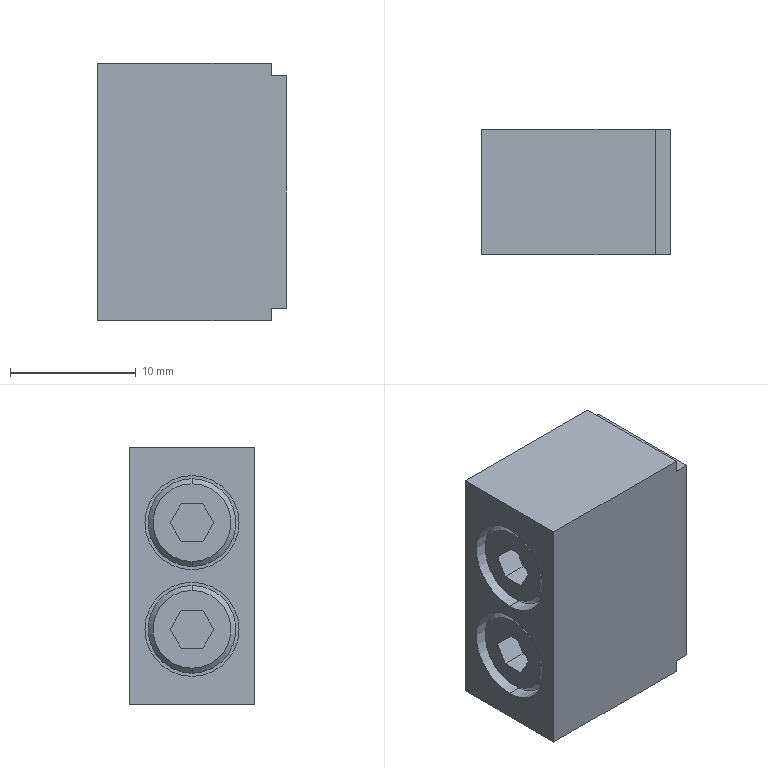Part | SolidWorks | features BaseBody 1 | 1 solid | 40 faces | box 15 x 10 x 20.5 mm | volume 2936 mm3 | plane 28 | cylinder 8 | cone 4 | commonest cylinder face diameters 7 x4 7.5 x4
STEP:
#1=CARTESIAN_POINT('',(-14.6,0.,7.35));
#2=VERTEX_POINT('',#1);
#3=CARTESIAN_POINT('',(-14.6,0.,1.15));
#4=VERTEX_POINT('',#3);
#5=CARTESIAN_POINT('',(-14.6,0.,4.25));
#6=DIRECTION('',(-1.,0.,0.));
#7=DIRECTION('',(0.,0.,1.));
#8=AXIS2_PLACEMENT_3D('',#5,#6,#7);
#9=CIRCLE('',#8,3.1);
#10=EDGE_CURVE('',#2,#4,#9,.T.);
#11=ORIENTED_EDGE('',*,*,#10,.F.);
#12=CARTESIAN_POINT('',(-14.2,0.,7.75));
#13=VERTEX_POINT('',#12);
#14=CARTESIAN_POINT('',(-14.2,0.,7.75));
#15=DIRECTION('',(0.7071,0.,0.7071));
#16=VECTOR('',#15,1000.);
#17=LINE('',#14,#16);
#18=EDGE_CURVE('',#2,#13,#17,.T.);
#19=ORIENTED_EDGE('',*,*,#18,.T.);
#20=CARTESIAN_POINT('',(-14.2,0.,0.75));
#21=VERTEX_POINT('',#20);
#22=CARTESIAN_POINT('',(-14.2,0.,4.25));
#23=DIRECTION('',(-1.,0.,0.));
#24=DIRECTION('',(0.,0.,1.));
#25=AXIS2_PLACEMENT_3D('',#22,#23,#24);
#26=CIRCLE('',#25,3.5);
#27=EDGE_CURVE('',#13,#21,#26,.T.);
#28=ORIENTED_EDGE('',*,*,#27,.T.);
#29=CARTESIAN_POINT('',(-14.2,0.,0.75));
#30=DIRECTION('',(0.7071,0.,-0.7071));
#31=VECTOR('',#30,1000.);
#32=LINE('',#29,#31);
#33=EDGE_CURVE('',#4,#21,#32,.T.);
#34=ORIENTED_EDGE('',*,*,#33,.F.);
#35=EDGE_LOOP('',(#11,#19,#28,#34));
#36=FACE_OUTER_BOUND('',#35,.T.);
#37=CARTESIAN_POINT('',(-14.2,0.,4.25));
#38=DIRECTION('',(1.,0.,0.));
#39=DIRECTION('',(0.,0.,-1.));
#40=AXIS2_PLACEMENT_3D('',#37,#38,#39);
#41=CONICAL_SURFACE('',#40,3.5,0.7854);
#42=ADVANCED_FACE('',(#36),#41,.T.);
#43=CARTESIAN_POINT('',(-10.6,0.,7.75));
#44=VERTEX_POINT('',#43);
#45=CARTESIAN_POINT('',(-10.6,0.,0.75));
#46=VERTEX_POINT('',#45);
#47=CARTESIAN_POINT('',(-10.6,0.,4.25));
#48=DIRECTION('',(-1.,0.,0.));
#49=DIRECTION('',(0.,0.,-1.));
#50=AXIS2_PLACEMENT_3D('',#47,#48,#49);
#51=CIRCLE('',#50,3.5);
#52=EDGE_CURVE('',#44,#46,#51,.T.);
#53=ORIENTED_EDGE('',*,*,#52,.T.);
#54=CARTESIAN_POINT('',(-14.6,0.,0.75));
#55=DIRECTION('',(-1.,0.,0.));
#56=VECTOR('',#55,1000.);
#57=LINE('',#54,#56);
#58=EDGE_CURVE('',#46,#21,#57,.T.);
#59=ORIENTED_EDGE('',*,*,#58,.T.);
#60=ORIENTED_EDGE('',*,*,#27,.F.);
#61=CARTESIAN_POINT('',(-14.6,0.,7.75));
#62=DIRECTION('',(-1.,0.,0.));
#63=VECTOR('',#62,1000.);
#64=LINE('',#61,#63);
#65=EDGE_CURVE('',#44,#13,#64,.T.);
#66=ORIENTED_EDGE('',*,*,#65,.F.);
#67=EDGE_LOOP('',(#53,#59,#60,#66));
#68=FACE_OUTER_BOUND('',#67,.T.);
#69=CARTESIAN_POINT('',(-14.6,0.,4.25));
#70=DIRECTION('',(-1.,0.,0.));
#71=DIRECTION('',(0.,0.,1.));
#72=AXIS2_PLACEMENT_3D('',#69,#70,#71);
#73=CYLINDRICAL_SURFACE('',#72,3.5);
#74=ADVANCED_FACE('',(#68),#73,.T.);
#75=CARTESIAN_POINT('',(-10.6,0.,8.));
#76=VERTEX_POINT('',#75);
#77=CARTESIAN_POINT('',(-10.6,0.,0.5));
#78=VERTEX_POINT('',#77);
#79=CARTESIAN_POINT('',(-10.6,0.,4.25));
#80=DIRECTION('',(1.,0.,0.));
#81=DIRECTION('',(0.,0.,-1.));
#82=AXIS2_PLACEMENT_3D('',#79,#80,#81);
#83=CIRCLE('',#82,3.75);
#84=EDGE_CURVE('',#76,#78,#83,.T.);
#85=ORIENTED_EDGE('',*,*,#84,.T.);
#86=CARTESIAN_POINT('',(-15.,0.,0.5));
#87=VERTEX_POINT('',#86);
#88=CARTESIAN_POINT('',(-10.6,0.,0.5));
#89=DIRECTION('',(-1.,0.,0.));
#90=VECTOR('',#89,1000.);
#91=LINE('',#88,#90);
#92=EDGE_CURVE('',#78,#87,#91,.T.);
#93=ORIENTED_EDGE('',*,*,#92,.T.);
#94=CARTESIAN_POINT('',(-15.,0.,8.));
#95=VERTEX_POINT('',#94);
#96=CARTESIAN_POINT('',(-15.,0.,4.25));
#97=DIRECTION('',(1.,0.,0.));
#98=DIRECTION('',(0.,0.,-1.));
#99=AXIS2_PLACEMENT_3D('',#96,#97,#98);
#100=CIRCLE('',#99,3.75);
#101=EDGE_CURVE('',#95,#87,#100,.T.);
#102=ORIENTED_EDGE('',*,*,#101,.F.);
#103=CARTESIAN_POINT('',(-10.6,0.,8.));
#104=DIRECTION('',(-1.,0.,0.));
#105=VECTOR('',#104,1000.);
#106=LINE('',#103,#105);
#107=EDGE_CURVE('',#76,#95,#106,.T.);
#108=ORIENTED_EDGE('',*,*,#107,.F.);
#109=EDGE_LOOP('',(#85,#93,#102,#108));
#110=FACE_OUTER_BOUND('',#109,.T.);
#111=CARTESIAN_POINT('',(-10.6,0.,4.25));
#112=DIRECTION('',(-1.,0.,0.));
#113=DIRECTION('',(0.,0.,1.));
#114=AXIS2_PLACEMENT_3D('',#111,#112,#113);
#115=CYLINDRICAL_SURFACE('',#114,3.75);
#116=ADVANCED_FACE('',(#110),#115,.F.);
#117=CARTESIAN_POINT('',(-10.6,0.,-0.5));
#118=VERTEX_POINT('',#117);
#119=CARTESIAN_POINT('',(-10.6,0.,-8.));
#120=VERTEX_POINT('',#119);
#121=CARTESIAN_POINT('',(-10.6,0.,-4.25));
#122=DIRECTION('',(1.,0.,0.));
#123=DIRECTION('',(0.,0.,-1.));
#124=AXIS2_PLACEMENT_3D('',#121,#122,#123);
#125=CIRCLE('',#124,3.75);
#126=EDGE_CURVE('',#118,#120,#125,.T.);
#127=ORIENTED_EDGE('',*,*,#126,.T.);
#128=CARTESIAN_POINT('',(-15.,0.,-8.));
#129=VERTEX_POINT('',#128);
#130=CARTESIAN_POINT('',(-10.6,0.,-8.));
#131=DIRECTION('',(-1.,0.,0.));
#132=VECTOR('',#131,1000.);
#133=LINE('',#130,#132);
#134=EDGE_CURVE('',#120,#129,#133,.T.);
#135=ORIENTED_EDGE('',*,*,#134,.T.);
#136=CARTESIAN_POINT('',(-15.,0.,-0.5));
#137=VERTEX_POINT('',#136);
#138=CARTESIAN_POINT('',(-15.,0.,-4.25));
#139=DIRECTION('',(1.,0.,0.));
#140=DIRECTION('',(0.,0.,-1.));
#141=AXIS2_PLACEMENT_3D('',#138,#139,#140);
#142=CIRCLE('',#141,3.75);
#143=EDGE_CURVE('',#137,#129,#142,.T.);
#144=ORIENTED_EDGE('',*,*,#143,.F.);
#145=CARTESIAN_POINT('',(-10.6,0.,-0.5));
#146=DIRECTION('',(-1.,0.,0.));
#147=VECTOR('',#146,1000.);
#148=LINE('',#145,#147);
#149=EDGE_CURVE('',#118,#137,#148,.T.);
#150=ORIENTED_EDGE('',*,*,#149,.F.);
#151=EDGE_LOOP('',(#127,#135,#144,#150));
#152=FACE_OUTER_BOUND('',#151,.T.);
#153=CARTESIAN_POINT('',(-10.6,0.,-4.25));
#154=DIRECTION('',(-1.,0.,0.));
#155=DIRECTION('',(0.,0.,1.));
#156=AXIS2_PLACEMENT_3D('',#153,#154,#155);
#157=CYLINDRICAL_SURFACE('',#156,3.75);
#158=ADVANCED_FACE('',(#152),#157,.F.);
#159=CARTESIAN_POINT('',(-10.6,0.,-0.75));
#160=VERTEX_POINT('',#159);
#161=CARTESIAN_POINT('',(-10.6,0.,-7.75));
#162=VERTEX_POINT('',#161);
#163=CARTESIAN_POINT('',(-10.6,0.,-4.25));
#164=DIRECTION('',(-1.,0.,0.));
#165=DIRECTION('',(0.,0.,-1.));
#166=AXIS2_PLACEMENT_3D('',#163,#164,#165);
#167=CIRCLE('',#166,3.5);
#168=EDGE_CURVE('',#160,#162,#167,.T.);
#169=ORIENTED_EDGE('',*,*,#168,.T.);
#170=CARTESIAN_POINT('',(-14.2,0.,-7.75));
#171=VERTEX_POINT('',#170);
#172=CARTESIAN_POINT('',(-14.6,0.,-7.75));
#173=DIRECTION('',(-1.,0.,0.));
#174=VECTOR('',#173,1000.);
#175=LINE('',#172,#174);
#176=EDGE_CURVE('',#162,#171,#175,.T.);
#177=ORIENTED_EDGE('',*,*,#176,.T.);
#178=CARTESIAN_POINT('',(-14.2,0.,-0.75));
#179=VERTEX_POINT('',#178);
#180=CARTESIAN_POINT('',(-14.2,0.,-4.25));
#181=DIRECTION('',(-1.,0.,0.));
#182=DIRECTION('',(0.,0.,1.));
#183=AXIS2_PLACEMENT_3D('',#180,#181,#182);
#184=CIRCLE('',#183,3.5);
#185=EDGE_CURVE('',#179,#171,#184,.T.);
#186=ORIENTED_EDGE('',*,*,#185,.F.);
#187=CARTESIAN_POINT('',(-14.6,0.,-0.75));
#188=DIRECTION('',(-1.,0.,0.));
#189=VECTOR('',#188,1000.);
#190=LINE('',#187,#189);
#191=EDGE_CURVE('',#160,#179,#190,.T.);
#192=ORIENTED_EDGE('',*,*,#191,.F.);
#193=EDGE_LOOP('',(#169,#177,#186,#192));
#194=FACE_OUTER_BOUND('',#193,.T.);
#195=CARTESIAN_POINT('',(-14.6,0.,-4.25));
#196=DIRECTION('',(-1.,0.,0.));
#197=DIRECTION('',(0.,0.,1.));
#198=AXIS2_PLACEMENT_3D('',#195,#196,#197);
#199=CYLINDRICAL_SURFACE('',#198,3.5);
#200=ADVANCED_FACE('',(#194),#199,.T.);
#201=CARTESIAN_POINT('',(-14.6,0.,-1.15));
#202=VERTEX_POINT('',#201);
#203=CARTESIAN_POINT('',(-14.6,0.,-7.35));
#204=VERTEX_POINT('',#203);
#205=CARTESIAN_POINT('',(-14.6,0.,-4.25));
#206=DIRECTION('',(-1.,0.,0.));
#207=DIRECTION('',(0.,0.,1.));
#208=AXIS2_PLACEMENT_3D('',#205,#206,#207);
#209=CIRCLE('',#208,3.1);
#210=EDGE_CURVE('',#202,#204,#209,.T.);
#211=ORIENTED_EDGE('',*,*,#210,.F.);
#212=CARTESIAN_POINT('',(-14.2,0.,-0.75));
#213=DIRECTION('',(0.7071,0.,0.7071));
#214=VECTOR('',#213,1000.);
#215=LINE('',#212,#214);
#216=EDGE_CURVE('',#202,#179,#215,.T.);
#217=ORIENTED_EDGE('',*,*,#216,.T.);
#218=ORIENTED_EDGE('',*,*,#185,.T.);
#219=CARTESIAN_POINT('',(-14.2,0.,-7.75));
#220=DIRECTION('',(0.7071,0.,-0.7071));
#221=VECTOR('',#220,1000.);
#222=LINE('',#219,#221);
#223=EDGE_CURVE('',#204,#171,#222,.T.);
#224=ORIENTED_EDGE('',*,*,#223,.F.);
#225=EDGE_LOOP('',(#211,#217,#218,#224));
#226=FACE_OUTER_BOUND('',#225,.T.);
#227=CARTESIAN_POINT('',(-14.2,0.,-4.25));
#228=DIRECTION('',(1.,0.,0.));
#229=DIRECTION('',(0.,0.,-1.));
#230=AXIS2_PLACEMENT_3D('',#227,#228,#229);
#231=CONICAL_SURFACE('',#230,3.5,0.7854);
#232=ADVANCED_FACE('',(#226),#231,.T.);
#233=CARTESIAN_POINT('',(-14.6,1.732,-4.25));
#234=VERTEX_POINT('',#233);
#235=CARTESIAN_POINT('',(-14.6,0.866,-2.75));
#236=VERTEX_POINT('',#235);
#237=CARTESIAN_POINT('',(-14.6,1.732,-4.25));
#238=DIRECTION('',(0.,-0.5,0.866));
#239=VECTOR('',#238,1000.);
#240=LINE('',#237,#239);
#241=EDGE_CURVE('',#234,#236,#240,.T.);
#242=ORIENTED_EDGE('',*,*,#241,.T.);
#243=CARTESIAN_POINT('',(-14.6,-0.866,-2.75));
#244=VERTEX_POINT('',#243);
#245=CARTESIAN_POINT('',(-14.6,-0.866,-2.75));
#246=DIRECTION('',(0.,1.,0.));
#247=VECTOR('',#246,1000.);
#248=LINE('',#245,#247);
#249=EDGE_CURVE('',#244,#236,#248,.T.);
#250=ORIENTED_EDGE('',*,*,#249,.F.);
#251=CARTESIAN_POINT('',(-14.6,-1.732,-4.25));
#252=VERTEX_POINT('',#251);
#253=CARTESIAN_POINT('',(-14.6,-0.866,-2.75));
#254=DIRECTION('',(0.,-0.5,-0.866));
#255=VECTOR('',#254,1000.);
#256=LINE('',#253,#255);
#257=EDGE_CURVE('',#244,#252,#256,.T.);
#258=ORIENTED_EDGE('',*,*,#257,.T.);
#259=CARTESIAN_POINT('',(-14.6,-0.866,-5.75));
#260=VERTEX_POINT('',#259);
#261=CARTESIAN_POINT('',(-14.6,-1.732,-4.25));
#262=DIRECTION('',(0.,0.5,-0.866));
#263=VECTOR('',#262,1000.);
#264=LINE('',#261,#263);
#265=EDGE_CURVE('',#252,#260,#264,.T.);
#266=ORIENTED_EDGE('',*,*,#265,.T.);
#267=CARTESIAN_POINT('',(-14.6,0.866,-5.75));
#268=VERTEX_POINT('',#267);
#269=CARTESIAN_POINT('',(-14.6,-0.866,-5.75));
#270=DIRECTION('',(0.,1.,0.));
#271=VECTOR('',#270,1000.);
#272=LINE('',#269,#271);
#273=EDGE_CURVE('',#260,#268,#272,.T.);
#274=ORIENTED_EDGE('',*,*,#273,.T.);
#275=CARTESIAN_POINT('',(-14.6,0.866,-5.75));
#276=DIRECTION('',(0.,0.5,0.866));
#277=VECTOR('',#276,1000.);
#278=LINE('',#275,#277);
#279=EDGE_CURVE('',#268,#234,#278,.T.);
#280=ORIENTED_EDGE('',*,*,#279,.T.);
#281=EDGE_LOOP('',(#242,#250,#258,#266,#274,#280));
#282=FACE_BOUND('',#281,.T.);
#283=CARTESIAN_POINT('',(-14.6,0.,-4.25));
#284=DIRECTION('',(-1.,0.,0.));
#285=DIRECTION('',(0.,0.,1.));
#286=AXIS2_PLACEMENT_3D('',#283,#284,#285);
#287=CIRCLE('',#286,3.1);
#288=EDGE_CURVE('',#204,#202,#287,.T.);
#289=ORIENTED_EDGE('',*,*,#288,.T.);
#290=ORIENTED_EDGE('',*,*,#210,.T.);
#291=EDGE_LOOP('',(#289,#290));
#292=FACE_OUTER_BOUND('',#291,.T.);
#293=CARTESIAN_POINT('',(-14.6,0.,-1.15));
#294=DIRECTION('',(1.,0.,0.));
#295=DIRECTION('',(0.,0.,-1.));
#296=AXIS2_PLACEMENT_3D('',#293,#294,#295);
#297=PLANE('',#296);
#298=ADVANCED_FACE('',(#282,#292),#297,.F.);
#299=ORIENTED_EDGE('',*,*,#241,.F.);
#300=CARTESIAN_POINT('',(-12.6,1.732,-4.25));
#301=VERTEX_POINT('',#300);
#302=CARTESIAN_POINT('',(-12.6,1.732,-4.25));
#303=DIRECTION('',(-1.,0.,0.));
#304=VECTOR('',#303,1000.);
#305=LINE('',#302,#304);
#306=EDGE_CURVE('',#301,#234,#305,.T.);
#307=ORIENTED_EDGE('',*,*,#306,.F.);
#308=CARTESIAN_POINT('',(-12.6,0.866,-2.75));
#309=VERTEX_POINT('',#308);
#310=CARTESIAN_POINT('',(-12.6,1.732,-4.25));
#311=DIRECTION('',(0.,-0.5,0.866));
#312=VECTOR('',#311,1000.);
#313=LINE('',#310,#312);
#314=EDGE_CURVE('',#301,#309,#313,.T.);
#315=ORIENTED_EDGE('',*,*,#314,.T.);
#316=CARTESIAN_POINT('',(-12.6,0.866,-2.75));
#317=DIRECTION('',(-1.,0.,0.));
#318=VECTOR('',#317,1000.);
#319=LINE('',#316,#318);
#320=EDGE_CURVE('',#309,#236,#319,.T.);
#321=ORIENTED_EDGE('',*,*,#320,.T.);
#322=EDGE_LOOP('',(#299,#307,#315,#321));
#323=FACE_OUTER_BOUND('',#322,.T.);
#324=CARTESIAN_POINT('',(-12.6,1.732,-4.25));
#325=DIRECTION('',(0.,-0.866,-0.5));
#326=DIRECTION('',(0.,0.5,-0.866));
#327=AXIS2_PLACEMENT_3D('',#324,#325,#326);
#328=PLANE('',#327);
#329=ADVANCED_FACE('',(#323),#328,.T.);
#330=ORIENTED_EDGE('',*,*,#249,.T.);
#331=ORIENTED_EDGE('',*,*,#320,.F.);
#332=CARTESIAN_POINT('',(-12.6,-0.866,-2.75));
#333=VERTEX_POINT('',#332);
#334=CARTESIAN_POINT('',(-12.6,0.866,-2.75));
#335=DIRECTION('',(0.,-1.,0.));
#336=VECTOR('',#335,1000.);
#337=LINE('',#334,#336);
#338=EDGE_CURVE('',#309,#333,#337,.T.);
#339=ORIENTED_EDGE('',*,*,#338,.T.);
#340=CARTESIAN_POINT('',(-12.6,-0.866,-2.75));
#341=DIRECTION('',(-1.,0.,0.));
#342=VECTOR('',#341,1000.);
#343=LINE('',#340,#342);
#344=EDGE_CURVE('',#333,#244,#343,.T.);
#345=ORIENTED_EDGE('',*,*,#344,.T.);
#346=EDGE_LOOP('',(#330,#331,#339,#345));
#347=FACE_OUTER_BOUND('',#346,.T.);
#348=CARTESIAN_POINT('',(-12.6,0.866,-2.75));
#349=DIRECTION('',(0.,0.,-1.));
#350=DIRECTION('',(-1.,0.,0.));
#351=AXIS2_PLACEMENT_3D('',#348,#349,#350);
#352=PLANE('',#351);
#353=ADVANCED_FACE('',(#347),#352,.T.);
#354=ORIENTED_EDGE('',*,*,#257,.F.);
#355=ORIENTED_EDGE('',*,*,#344,.F.);
#356=CARTESIAN_POINT('',(-12.6,-1.732,-4.25));
#357=VERTEX_POINT('',#356);
#358=CARTESIAN_POINT('',(-12.6,-0.866,-2.75));
#359=DIRECTION('',(0.,-0.5,-0.866));
#360=VECTOR('',#359,1000.);
#361=LINE('',#358,#360);
#362=EDGE_CURVE('',#333,#357,#361,.T.);
#363=ORIENTED_EDGE('',*,*,#362,.T.);
#364=CARTESIAN_POINT('',(-12.6,-1.732,-4.25));
#365=DIRECTION('',(-1.,0.,0.));
#366=VECTOR('',#365,1000.);
#367=LINE('',#364,#366);
#368=EDGE_CURVE('',#357,#252,#367,.T.);
#369=ORIENTED_EDGE('',*,*,#368,.T.);
#370=EDGE_LOOP('',(#354,#355,#363,#369));
#371=FACE_OUTER_BOUND('',#370,.T.);
#372=CARTESIAN_POINT('',(-12.6,-0.866,-2.75));
#373=DIRECTION('',(0.,0.866,-0.5));
#374=DIRECTION('',(0.,0.5,0.866));
#375=AXIS2_PLACEMENT_3D('',#372,#373,#374);
#376=PLANE('',#375);
#377=ADVANCED_FACE('',(#371),#376,.T.);
#378=ORIENTED_EDGE('',*,*,#265,.F.);
#379=ORIENTED_EDGE('',*,*,#368,.F.);
#380=CARTESIAN_POINT('',(-12.6,-0.866,-5.75));
#381=VERTEX_POINT('',#380);
#382=CARTESIAN_POINT('',(-12.6,-1.732,-4.25));
#383=DIRECTION('',(0.,0.5,-0.866));
#384=VECTOR('',#383,1000.);
#385=LINE('',#382,#384);
#386=EDGE_CURVE('',#357,#381,#385,.T.);
#387=ORIENTED_EDGE('',*,*,#386,.T.);
#388=CARTESIAN_POINT('',(-12.6,-0.866,-5.75));
#389=DIRECTION('',(-1.,0.,0.));
#390=VECTOR('',#389,1000.);
#391=LINE('',#388,#390);
#392=EDGE_CURVE('',#381,#260,#391,.T.);
#393=ORIENTED_EDGE('',*,*,#392,.T.);
#394=EDGE_LOOP('',(#378,#379,#387,#393));
#395=FACE_OUTER_BOUND('',#394,.T.);
#396=CARTESIAN_POINT('',(-12.6,-1.732,-4.25));
#397=DIRECTION('',(0.,0.866,0.5));
#398=DIRECTION('',(0.,-0.5,0.866));
#399=AXIS2_PLACEMENT_3D('',#396,#397,#398);
#400=PLANE('',#399);
#401=ADVANCED_FACE('',(#395),#400,.T.);
#402=ORIENTED_EDGE('',*,*,#273,.F.);
#403=ORIENTED_EDGE('',*,*,#392,.F.);
#404=CARTESIAN_POINT('',(-12.6,0.866,-5.75));
#405=VERTEX_POINT('',#404);
#406=CARTESIAN_POINT('',(-12.6,-0.866,-5.75));
#407=DIRECTION('',(0.,1.,0.));
#408=VECTOR('',#407,1000.);
#409=LINE('',#406,#408);
#410=EDGE_CURVE('',#381,#405,#409,.T.);
#411=ORIENTED_EDGE('',*,*,#410,.T.);
#412=CARTESIAN_POINT('',(-12.6,0.866,-5.75));
#413=DIRECTION('',(-1.,0.,0.));
#414=VECTOR('',#413,1000.);
#415=LINE('',#412,#414);
#416=EDGE_CURVE('',#405,#268,#415,.T.);
#417=ORIENTED_EDGE('',*,*,#416,.T.);
#418=EDGE_LOOP('',(#402,#403,#411,#417));
#419=FACE_OUTER_BOUND('',#418,.T.);
#420=CARTESIAN_POINT('',(-12.6,-0.866,-5.75));
#421=DIRECTION('',(0.,0.,1.));
#422=DIRECTION('',(1.,0.,0.));
#423=AXIS2_PLACEMENT_3D('',#420,#421,#422);
#424=PLANE('',#423);
#425=ADVANCED_FACE('',(#419),#424,.T.);
#426=ORIENTED_EDGE('',*,*,#279,.F.);
#427=ORIENTED_EDGE('',*,*,#416,.F.);
#428=CARTESIAN_POINT('',(-12.6,0.866,-5.75));
#429=DIRECTION('',(0.,0.5,0.866));
#430=VECTOR('',#429,1000.);
#431=LINE('',#428,#430);
#432=EDGE_CURVE('',#405,#301,#431,.T.);
#433=ORIENTED_EDGE('',*,*,#432,.T.);
#434=ORIENTED_EDGE('',*,*,#306,.T.);
#435=EDGE_LOOP('',(#426,#427,#433,#434));
#436=FACE_OUTER_BOUND('',#435,.T.);
#437=CARTESIAN_POINT('',(-12.6,0.866,-5.75));
#438=DIRECTION('',(0.,-0.866,0.5));
#439=DIRECTION('',(0.,-0.5,-0.866));
#440=AXIS2_PLACEMENT_3D('',#437,#438,#439);
#441=PLANE('',#440);
#442=ADVANCED_FACE('',(#436),#441,.T.);
#443=ORIENTED_EDGE('',*,*,#216,.F.);
#444=ORIENTED_EDGE('',*,*,#288,.F.);
#445=ORIENTED_EDGE('',*,*,#223,.T.);
#446=CARTESIAN_POINT('',(-14.2,0.,-4.25));
#447=DIRECTION('',(-1.,0.,0.));
#448=DIRECTION('',(0.,0.,1.));
#449=AXIS2_PLACEMENT_3D('',#446,#447,#448);
#450=CIRCLE('',#449,3.5);
#451=EDGE_CURVE('',#171,#179,#450,.T.);
#452=ORIENTED_EDGE('',*,*,#451,.T.);
#453=EDGE_LOOP('',(#443,#444,#445,#452));
#454=FACE_OUTER_BOUND('',#453,.T.);
#455=CARTESIAN_POINT('',(-14.2,0.,-4.25));
#456=DIRECTION('',(1.,0.,0.));
#457=DIRECTION('',(0.,0.,-1.));
#458=AXIS2_PLACEMENT_3D('',#455,#456,#457);
#459=CONICAL_SURFACE('',#458,3.5,0.7854);
#460=ADVANCED_FACE('',(#454),#459,.T.);
#461=ORIENTED_EDGE('',*,*,#338,.F.);
#462=ORIENTED_EDGE('',*,*,#314,.F.);
#463=ORIENTED_EDGE('',*,*,#432,.F.);
#464=ORIENTED_EDGE('',*,*,#410,.F.);
#465=ORIENTED_EDGE('',*,*,#386,.F.);
#466=ORIENTED_EDGE('',*,*,#362,.F.);
#467=EDGE_LOOP('',(#461,#462,#463,#464,#465,#466));
#468=FACE_OUTER_BOUND('',#467,.T.);
#469=CARTESIAN_POINT('',(-12.6,0.,-8.5));
#470=DIRECTION('',(1.,0.,0.));
#471=DIRECTION('',(0.,0.,-1.));
#472=AXIS2_PLACEMENT_3D('',#469,#470,#471);
#473=PLANE('',#472);
#474=ADVANCED_FACE('',(#468),#473,.F.);
#475=ORIENTED_EDGE('',*,*,#176,.F.);
#476=CARTESIAN_POINT('',(-10.6,0.,-4.25));
#477=DIRECTION('',(-1.,0.,0.));
#478=DIRECTION('',(0.,0.,-1.));
#479=AXIS2_PLACEMENT_3D('',#476,#477,#478);
#480=CIRCLE('',#479,3.5);
#481=EDGE_CURVE('',#162,#160,#480,.T.);
#482=ORIENTED_EDGE('',*,*,#481,.T.);
#483=ORIENTED_EDGE('',*,*,#191,.T.);
#484=ORIENTED_EDGE('',*,*,#451,.F.);
#485=EDGE_LOOP('',(#475,#482,#483,#484));
#486=FACE_OUTER_BOUND('',#485,.T.);
#487=CARTESIAN_POINT('',(-14.6,0.,-4.25));
#488=DIRECTION('',(-1.,0.,0.));
#489=DIRECTION('',(0.,0.,1.));
#490=AXIS2_PLACEMENT_3D('',#487,#488,#489);
#491=CYLINDRICAL_SURFACE('',#490,3.5);
#492=ADVANCED_FACE('',(#486),#491,.T.);
#493=ORIENTED_EDGE('',*,*,#168,.F.);
#494=ORIENTED_EDGE('',*,*,#481,.F.);
#495=EDGE_LOOP('',(#493,#494));
#496=FACE_BOUND('',#495,.T.);
#497=ORIENTED_EDGE('',*,*,#126,.F.);
#498=CARTESIAN_POINT('',(-10.6,0.,-4.25));
#499=DIRECTION('',(1.,0.,0.));
#500=DIRECTION('',(0.,0.,-1.));
#501=AXIS2_PLACEMENT_3D('',#498,#499,#500);
#502=CIRCLE('',#501,3.75);
#503=EDGE_CURVE('',#120,#118,#502,.T.);
#504=ORIENTED_EDGE('',*,*,#503,.F.);
#505=EDGE_LOOP('',(#497,#504));
#506=FACE_OUTER_BOUND('',#505,.T.);
#507=CARTESIAN_POINT('',(-10.6,0.,-4.25));
#508=DIRECTION('',(1.,0.,0.));
#509=DIRECTION('',(0.,0.,-1.));
#510=AXIS2_PLACEMENT_3D('',#507,#508,#509);
#511=PLANE('',#510);
#512=ADVANCED_FACE('',(#496,#506),#511,.F.);
#513=ORIENTED_EDGE('',*,*,#134,.F.);
#514=ORIENTED_EDGE('',*,*,#503,.T.);
#515=ORIENTED_EDGE('',*,*,#149,.T.);
#516=CARTESIAN_POINT('',(-15.,0.,-4.25));
#517=DIRECTION('',(1.,0.,0.));
#518=DIRECTION('',(0.,0.,-1.));
#519=AXIS2_PLACEMENT_3D('',#516,#517,#518);
#520=CIRCLE('',#519,3.75);
#521=EDGE_CURVE('',#129,#137,#520,.T.);
#522=ORIENTED_EDGE('',*,*,#521,.F.);
#523=EDGE_LOOP('',(#513,#514,#515,#522));
#524=FACE_OUTER_BOUND('',#523,.T.);
#525=CARTESIAN_POINT('',(-10.6,0.,-4.25));
#526=DIRECTION('',(-1.,0.,0.));
#527=DIRECTION('',(0.,0.,1.));
#528=AXIS2_PLACEMENT_3D('',#525,#526,#527);
#529=CYLINDRICAL_SURFACE('',#528,3.75);
#530=ADVANCED_FACE('',(#524),#529,.F.);
#531=ORIENTED_EDGE('',*,*,#143,.T.);
#532=ORIENTED_EDGE('',*,*,#521,.T.);
#533=EDGE_LOOP('',(#531,#532));
#534=FACE_BOUND('',#533,.T.);
#535=ORIENTED_EDGE('',*,*,#101,.T.);
#536=CARTESIAN_POINT('',(-15.,0.,4.25));
#537=DIRECTION('',(1.,0.,0.));
#538=DIRECTION('',(0.,0.,-1.));
#539=AXIS2_PLACEMENT_3D('',#536,#537,#538);
#540=CIRCLE('',#539,3.75);
#541=EDGE_CURVE('',#87,#95,#540,.T.);
#542=ORIENTED_EDGE('',*,*,#541,.T.);
#543=EDGE_LOOP('',(#535,#542));
#544=FACE_BOUND('',#543,.T.);
#545=CARTESIAN_POINT('',(-15.,-5.,-10.25));
#546=VERTEX_POINT('',#545);
#547=CARTESIAN_POINT('',(-15.,-5.,10.25));
#548=VERTEX_POINT('',#547);
#549=CARTESIAN_POINT('',(-15.,-5.,-10.25));
#550=DIRECTION('',(0.,0.,1.));
#551=VECTOR('',#550,1000.);
#552=LINE('',#549,#551);
#553=EDGE_CURVE('',#546,#548,#552,.T.);
#554=ORIENTED_EDGE('',*,*,#553,.T.);
#555=CARTESIAN_POINT('',(-15.,5.,10.25));
#556=VERTEX_POINT('',#555);
#557=CARTESIAN_POINT('',(-15.,5.,10.25));
#558=DIRECTION('',(0.,-1.,0.));
#559=VECTOR('',#558,1000.);
#560=LINE('',#557,#559);
#561=EDGE_CURVE('',#556,#548,#560,.T.);
#562=ORIENTED_EDGE('',*,*,#561,.F.);
#563=CARTESIAN_POINT('',(-15.,5.,-10.25));
#564=VERTEX_POINT('',#563);
#565=CARTESIAN_POINT('',(-15.,5.,-10.25));
#566=DIRECTION('',(0.,0.,1.));
#567=VECTOR('',#566,1000.);
#568=LINE('',#565,#567);
#569=EDGE_CURVE('',#564,#556,#568,.T.);
#570=ORIENTED_EDGE('',*,*,#569,.F.);
#571=CARTESIAN_POINT('',(-15.,5.,-10.25));
#572=DIRECTION('',(0.,-1.,0.));
#573=VECTOR('',#572,1000.);
#574=LINE('',#571,#573);
#575=EDGE_CURVE('',#564,#546,#574,.T.);
#576=ORIENTED_EDGE('',*,*,#575,.T.);
#577=EDGE_LOOP('',(#554,#562,#570,#576));
#578=FACE_OUTER_BOUND('',#577,.T.);
#579=CARTESIAN_POINT('',(-15.,5.,-10.25));
#580=DIRECTION('',(1.,0.,0.));
#581=DIRECTION('',(0.,0.,-1.));
#582=AXIS2_PLACEMENT_3D('',#579,#580,#581);
#583=PLANE('',#582);
#584=ADVANCED_FACE('',(#534,#544,#578),#583,.F.);
#585=ORIENTED_EDGE('',*,*,#92,.F.);
#586=CARTESIAN_POINT('',(-10.6,0.,4.25));
#587=DIRECTION('',(1.,0.,0.));
#588=DIRECTION('',(0.,0.,-1.));
#589=AXIS2_PLACEMENT_3D('',#586,#587,#588);
#590=CIRCLE('',#589,3.75);
#591=EDGE_CURVE('',#78,#76,#590,.T.);
#592=ORIENTED_EDGE('',*,*,#591,.T.);
#593=ORIENTED_EDGE('',*,*,#107,.T.);
#594=ORIENTED_EDGE('',*,*,#541,.F.);
#595=EDGE_LOOP('',(#585,#592,#593,#594));
#596=FACE_OUTER_BOUND('',#595,.T.);
#597=CARTESIAN_POINT('',(-10.6,0.,4.25));
#598=DIRECTION('',(-1.,0.,0.));
#599=DIRECTION('',(0.,0.,1.));
#600=AXIS2_PLACEMENT_3D('',#597,#598,#599);
#601=CYLINDRICAL_SURFACE('',#600,3.75);
#602=ADVANCED_FACE('',(#596),#601,.F.);
#603=CARTESIAN_POINT('',(-1.2,-5.,-10.25));
#604=VERTEX_POINT('',#603);
#605=CARTESIAN_POINT('',(-1.2,-5.,-10.25));
#606=DIRECTION('',(-1.,0.,0.));
#607=VECTOR('',#606,1000.);
#608=LINE('',#605,#607);
#609=EDGE_CURVE('',#604,#546,#608,.T.);
#610=ORIENTED_EDGE('',*,*,#609,.F.);
#611=CARTESIAN_POINT('',(-1.2,-5.,-9.25));
#612=VERTEX_POINT('',#611);
#613=CARTESIAN_POINT('',(-1.2,-5.,-9.25));
#614=DIRECTION('',(0.,0.,-1.));
#615=VECTOR('',#614,1000.);
#616=LINE('',#613,#615);
#617=EDGE_CURVE('',#612,#604,#616,.T.);
#618=ORIENTED_EDGE('',*,*,#617,.F.);
#619=CARTESIAN_POINT('',(0.,-5.,-9.25));
#620=VERTEX_POINT('',#619);
#621=CARTESIAN_POINT('',(0.,-5.,-9.25));
#622=DIRECTION('',(-1.,0.,0.));
#623=VECTOR('',#622,1000.);
#624=LINE('',#621,#623);
#625=EDGE_CURVE('',#620,#612,#624,.T.);
#626=ORIENTED_EDGE('',*,*,#625,.F.);
#627=CARTESIAN_POINT('',(0.,-5.,9.25));
#628=VERTEX_POINT('',#627);
#629=CARTESIAN_POINT('',(0.,-5.,9.25));
#630=DIRECTION('',(0.,0.,-1.));
#631=VECTOR('',#630,1000.);
#632=LINE('',#629,#631);
#633=EDGE_CURVE('',#628,#620,#632,.T.);
#634=ORIENTED_EDGE('',*,*,#633,.F.);
#635=CARTESIAN_POINT('',(-1.2,-5.,9.25));
#636=VERTEX_POINT('',#635);
#637=CARTESIAN_POINT('',(-1.2,-5.,9.25));
#638=DIRECTION('',(1.,0.,0.));
#639=VECTOR('',#638,1000.);
#640=LINE('',#637,#639);
#641=EDGE_CURVE('',#636,#628,#640,.T.);
#642=ORIENTED_EDGE('',*,*,#641,.F.);
#643=CARTESIAN_POINT('',(-1.2,-5.,10.25));
#644=VERTEX_POINT('',#643);
#645=CARTESIAN_POINT('',(-1.2,-5.,10.25));
#646=DIRECTION('',(0.,0.,-1.));
#647=VECTOR('',#646,1000.);
#648=LINE('',#645,#647);
#649=EDGE_CURVE('',#644,#636,#648,.T.);
#650=ORIENTED_EDGE('',*,*,#649,.F.);
#651=CARTESIAN_POINT('',(-15.,-5.,10.25));
#652=DIRECTION('',(1.,0.,0.));
#653=VECTOR('',#652,1000.);
#654=LINE('',#651,#653);
#655=EDGE_CURVE('',#548,#644,#654,.T.);
#656=ORIENTED_EDGE('',*,*,#655,.F.);
#657=ORIENTED_EDGE('',*,*,#553,.F.);
#658=EDGE_LOOP('',(#610,#618,#626,#634,#642,#650,#656,#657));
#659=FACE_OUTER_BOUND('',#658,.T.);
#660=CARTESIAN_POINT('',(0.,-5.,0.));
#661=DIRECTION('',(0.,1.,0.));
#662=DIRECTION('',(0.,0.,1.));
#663=AXIS2_PLACEMENT_3D('',#660,#661,#662);
#664=PLANE('',#663);
#665=ADVANCED_FACE('',(#659),#664,.F.);
#666=ORIENTED_EDGE('',*,*,#655,.T.);
#667=CARTESIAN_POINT('',(-1.2,5.,10.25));
#668=VERTEX_POINT('',#667);
#669=CARTESIAN_POINT('',(-1.2,5.,10.25));
#670=DIRECTION('',(0.,-1.,0.));
#671=VECTOR('',#670,1000.);
#672=LINE('',#669,#671);
#673=EDGE_CURVE('',#668,#644,#672,.T.);
#674=ORIENTED_EDGE('',*,*,#673,.F.);
#675=CARTESIAN_POINT('',(-15.,5.,10.25));
#676=DIRECTION('',(1.,0.,0.));
#677=VECTOR('',#676,1000.);
#678=LINE('',#675,#677);
#679=EDGE_CURVE('',#556,#668,#678,.T.);
#680=ORIENTED_EDGE('',*,*,#679,.F.);
#681=ORIENTED_EDGE('',*,*,#561,.T.);
#682=EDGE_LOOP('',(#666,#674,#680,#681));
#683=FACE_OUTER_BOUND('',#682,.T.);
#684=CARTESIAN_POINT('',(-15.,5.,10.25));
#685=DIRECTION('',(0.,0.,-1.));
#686=DIRECTION('',(-1.,0.,0.));
#687=AXIS2_PLACEMENT_3D('',#684,#685,#686);
#688=PLANE('',#687);
#689=ADVANCED_FACE('',(#683),#688,.F.);
#690=CARTESIAN_POINT('',(-1.2,5.,-10.25));
#691=VERTEX_POINT('',#690);
#692=CARTESIAN_POINT('',(-1.2,5.,-10.25));
#693=DIRECTION('',(-1.,0.,0.));
#694=VECTOR('',#693,1000.);
#695=LINE('',#692,#694);
#696=EDGE_CURVE('',#691,#564,#695,.T.);
#697=ORIENTED_EDGE('',*,*,#696,.T.);
#698=ORIENTED_EDGE('',*,*,#569,.T.);
#699=ORIENTED_EDGE('',*,*,#679,.T.);
#700=CARTESIAN_POINT('',(-1.2,5.,9.25));
#701=VERTEX_POINT('',#700);
#702=CARTESIAN_POINT('',(-1.2,5.,10.25));
#703=DIRECTION('',(0.,0.,-1.));
#704=VECTOR('',#703,1000.);
#705=LINE('',#702,#704);
#706=EDGE_CURVE('',#668,#701,#705,.T.);
#707=ORIENTED_EDGE('',*,*,#706,.T.);
#708=CARTESIAN_POINT('',(0.,5.,9.25));
#709=VERTEX_POINT('',#708);
#710=CARTESIAN_POINT('',(-1.2,5.,9.25));
#711=DIRECTION('',(1.,0.,0.));
#712=VECTOR('',#711,1000.);
#713=LINE('',#710,#712);
#714=EDGE_CURVE('',#701,#709,#713,.T.);
#715=ORIENTED_EDGE('',*,*,#714,.T.);
#716=CARTESIAN_POINT('',(0.,5.,-9.25));
#717=VERTEX_POINT('',#716);
#718=CARTESIAN_POINT('',(0.,5.,9.25));
#719=DIRECTION('',(0.,0.,-1.));
#720=VECTOR('',#719,1000.);
#721=LINE('',#718,#720);
#722=EDGE_CURVE('',#709,#717,#721,.T.);
#723=ORIENTED_EDGE('',*,*,#722,.T.);
#724=CARTESIAN_POINT('',(-1.2,5.,-9.25));
#725=VERTEX_POINT('',#724);
#726=CARTESIAN_POINT('',(0.,5.,-9.25));
#727=DIRECTION('',(-1.,0.,0.));
#728=VECTOR('',#727,1000.);
#729=LINE('',#726,#728);
#730=EDGE_CURVE('',#717,#725,#729,.T.);
#731=ORIENTED_EDGE('',*,*,#730,.T.);
#732=CARTESIAN_POINT('',(-1.2,5.,-9.25));
#733=DIRECTION('',(0.,0.,-1.));
#734=VECTOR('',#733,1000.);
#735=LINE('',#732,#734);
#736=EDGE_CURVE('',#725,#691,#735,.T.);
#737=ORIENTED_EDGE('',*,*,#736,.T.);
#738=EDGE_LOOP('',(#697,#698,#699,#707,#715,#723,#731,#737));
#739=FACE_OUTER_BOUND('',#738,.T.);
#740=CARTESIAN_POINT('',(0.,5.,0.));
#741=DIRECTION('',(0.,1.,0.));
#742=DIRECTION('',(0.,0.,1.));
#743=AXIS2_PLACEMENT_3D('',#740,#741,#742);
#744=PLANE('',#743);
#745=ADVANCED_FACE('',(#739),#744,.T.);
#746=ORIENTED_EDGE('',*,*,#609,.T.);
#747=ORIENTED_EDGE('',*,*,#575,.F.);
#748=ORIENTED_EDGE('',*,*,#696,.F.);
#749=CARTESIAN_POINT('',(-1.2,5.,-10.25));
#750=DIRECTION('',(0.,-1.,0.));
#751=VECTOR('',#750,1000.);
#752=LINE('',#749,#751);
#753=EDGE_CURVE('',#691,#604,#752,.T.);
#754=ORIENTED_EDGE('',*,*,#753,.T.);
#755=EDGE_LOOP('',(#746,#747,#748,#754));
#756=FACE_OUTER_BOUND('',#755,.T.);
#757=CARTESIAN_POINT('',(-1.2,5.,-10.25));
#758=DIRECTION('',(0.,0.,1.));
#759=DIRECTION('',(1.,0.,0.));
#760=AXIS2_PLACEMENT_3D('',#757,#758,#759);
#761=PLANE('',#760);
#762=ADVANCED_FACE('',(#756),#761,.F.);
#763=ORIENTED_EDGE('',*,*,#52,.F.);
#764=CARTESIAN_POINT('',(-10.6,0.,4.25));
#765=DIRECTION('',(-1.,0.,0.));
#766=DIRECTION('',(0.,0.,-1.));
#767=AXIS2_PLACEMENT_3D('',#764,#765,#766);
#768=CIRCLE('',#767,3.5);
#769=EDGE_CURVE('',#46,#44,#768,.T.);
#770=ORIENTED_EDGE('',*,*,#769,.F.);
#771=EDGE_LOOP('',(#763,#770));
#772=FACE_BOUND('',#771,.T.);
#773=ORIENTED_EDGE('',*,*,#84,.F.);
#774=ORIENTED_EDGE('',*,*,#591,.F.);
#775=EDGE_LOOP('',(#773,#774));
#776=FACE_OUTER_BOUND('',#775,.T.);
#777=CARTESIAN_POINT('',(-10.6,0.,4.25));
#778=DIRECTION('',(1.,0.,0.));
#779=DIRECTION('',(0.,0.,-1.));
#780=AXIS2_PLACEMENT_3D('',#777,#778,#779);
#781=PLANE('',#780);
#782=ADVANCED_FACE('',(#772,#776),#781,.F.);
#783=ORIENTED_EDGE('',*,*,#617,.T.);
#784=ORIENTED_EDGE('',*,*,#753,.F.);
#785=ORIENTED_EDGE('',*,*,#736,.F.);
#786=CARTESIAN_POINT('',(-1.2,5.,-9.25));
#787=DIRECTION('',(0.,-1.,0.));
#788=VECTOR('',#787,1000.);
#789=LINE('',#786,#788);
#790=EDGE_CURVE('',#725,#612,#789,.T.);
#791=ORIENTED_EDGE('',*,*,#790,.T.);
#792=EDGE_LOOP('',(#783,#784,#785,#791));
#793=FACE_OUTER_BOUND('',#792,.T.);
#794=CARTESIAN_POINT('',(-1.2,5.,-9.25));
#795=DIRECTION('',(-1.,0.,0.));
#796=DIRECTION('',(0.,0.,1.));
#797=AXIS2_PLACEMENT_3D('',#794,#795,#796);
#798=PLANE('',#797);
#799=ADVANCED_FACE('',(#793),#798,.F.);
#800=ORIENTED_EDGE('',*,*,#625,.T.);
#801=ORIENTED_EDGE('',*,*,#790,.F.);
#802=ORIENTED_EDGE('',*,*,#730,.F.);
#803=CARTESIAN_POINT('',(0.,5.,-9.25));
#804=DIRECTION('',(0.,-1.,0.));
#805=VECTOR('',#804,1000.);
#806=LINE('',#803,#805);
#807=EDGE_CURVE('',#717,#620,#806,.T.);
#808=ORIENTED_EDGE('',*,*,#807,.T.);
#809=EDGE_LOOP('',(#800,#801,#802,#808));
#810=FACE_OUTER_BOUND('',#809,.T.);
#811=CARTESIAN_POINT('',(0.,5.,-9.25));
#812=DIRECTION('',(0.,0.,1.));
#813=DIRECTION('',(1.,0.,0.));
#814=AXIS2_PLACEMENT_3D('',#811,#812,#813);
#815=PLANE('',#814);
#816=ADVANCED_FACE('',(#810),#815,.F.);
#817=ORIENTED_EDGE('',*,*,#633,.T.);
#818=ORIENTED_EDGE('',*,*,#807,.F.);
#819=ORIENTED_EDGE('',*,*,#722,.F.);
#820=CARTESIAN_POINT('',(0.,5.,9.25));
#821=DIRECTION('',(0.,-1.,0.));
#822=VECTOR('',#821,1000.);
#823=LINE('',#820,#822);
#824=EDGE_CURVE('',#709,#628,#823,.T.);
#825=ORIENTED_EDGE('',*,*,#824,.T.);
#826=EDGE_LOOP('',(#817,#818,#819,#825));
#827=FACE_OUTER_BOUND('',#826,.T.);
#828=CARTESIAN_POINT('',(0.,5.,9.25));
#829=DIRECTION('',(-1.,0.,0.));
#830=DIRECTION('',(0.,0.,1.));
#831=AXIS2_PLACEMENT_3D('',#828,#829,#830);
#832=PLANE('',#831);
#833=ADVANCED_FACE('',(#827),#832,.F.);
#834=ORIENTED_EDGE('',*,*,#641,.T.);
#835=ORIENTED_EDGE('',*,*,#824,.F.);
#836=ORIENTED_EDGE('',*,*,#714,.F.);
#837=CARTESIAN_POINT('',(-1.2,5.,9.25));
#838=DIRECTION('',(0.,-1.,0.));
#839=VECTOR('',#838,1000.);
#840=LINE('',#837,#839);
#841=EDGE_CURVE('',#701,#636,#840,.T.);
#842=ORIENTED_EDGE('',*,*,#841,.T.);
#843=EDGE_LOOP('',(#834,#835,#836,#842));
#844=FACE_OUTER_BOUND('',#843,.T.);
#845=CARTESIAN_POINT('',(-1.2,5.,9.25));
#846=DIRECTION('',(0.,0.,-1.));
#847=DIRECTION('',(-1.,0.,0.));
#848=AXIS2_PLACEMENT_3D('',#845,#846,#847);
#849=PLANE('',#848);
#850=ADVANCED_FACE('',(#844),#849,.F.);
#851=ORIENTED_EDGE('',*,*,#649,.T.);
#852=ORIENTED_EDGE('',*,*,#841,.F.);
#853=ORIENTED_EDGE('',*,*,#706,.F.);
#854=ORIENTED_EDGE('',*,*,#673,.T.);
#855=EDGE_LOOP('',(#851,#852,#853,#854));
#856=FACE_OUTER_BOUND('',#855,.T.);
#857=CARTESIAN_POINT('',(-1.2,5.,10.25));
#858=DIRECTION('',(-1.,0.,0.));
#859=DIRECTION('',(0.,0.,1.));
#860=AXIS2_PLACEMENT_3D('',#857,#858,#859);
#861=PLANE('',#860);
#862=ADVANCED_FACE('',(#856),#861,.F.);
#863=ORIENTED_EDGE('',*,*,#58,.F.);
#864=ORIENTED_EDGE('',*,*,#769,.T.);
#865=ORIENTED_EDGE('',*,*,#65,.T.);
#866=CARTESIAN_POINT('',(-14.2,0.,4.25));
#867=DIRECTION('',(-1.,0.,0.));
#868=DIRECTION('',(0.,0.,1.));
#869=AXIS2_PLACEMENT_3D('',#866,#867,#868);
#870=CIRCLE('',#869,3.5);
#871=EDGE_CURVE('',#21,#13,#870,.T.);
#872=ORIENTED_EDGE('',*,*,#871,.F.);
#873=EDGE_LOOP('',(#863,#864,#865,#872));
#874=FACE_OUTER_BOUND('',#873,.T.);
#875=CARTESIAN_POINT('',(-14.6,0.,4.25));
#876=DIRECTION('',(-1.,0.,0.));
#877=DIRECTION('',(0.,0.,1.));
#878=AXIS2_PLACEMENT_3D('',#875,#876,#877);
#879=CYLINDRICAL_SURFACE('',#878,3.5);
#880=ADVANCED_FACE('',(#874),#879,.T.);
#881=ORIENTED_EDGE('',*,*,#18,.F.);
#882=CARTESIAN_POINT('',(-14.6,0.,4.25));
#883=DIRECTION('',(-1.,0.,0.));
#884=DIRECTION('',(0.,0.,1.));
#885=AXIS2_PLACEMENT_3D('',#882,#883,#884);
#886=CIRCLE('',#885,3.1);
#887=EDGE_CURVE('',#4,#2,#886,.T.);
#888=ORIENTED_EDGE('',*,*,#887,.F.);
#889=ORIENTED_EDGE('',*,*,#33,.T.);
#890=ORIENTED_EDGE('',*,*,#871,.T.);
#891=EDGE_LOOP('',(#881,#888,#889,#890));
#892=FACE_OUTER_BOUND('',#891,.T.);
#893=CARTESIAN_POINT('',(-14.2,0.,4.25));
#894=DIRECTION('',(1.,0.,0.));
#895=DIRECTION('',(0.,0.,-1.));
#896=AXIS2_PLACEMENT_3D('',#893,#894,#895);
#897=CONICAL_SURFACE('',#896,3.5,0.7854);
#898=ADVANCED_FACE('',(#892),#897,.T.);
#899=CARTESIAN_POINT('',(-14.6,1.732,4.25));
#900=VERTEX_POINT('',#899);
#901=CARTESIAN_POINT('',(-14.6,0.866,5.75));
#902=VERTEX_POINT('',#901);
#903=CARTESIAN_POINT('',(-14.6,1.732,4.25));
#904=DIRECTION('',(0.,-0.5,0.866));
#905=VECTOR('',#904,1000.);
#906=LINE('',#903,#905);
#907=EDGE_CURVE('',#900,#902,#906,.T.);
#908=ORIENTED_EDGE('',*,*,#907,.T.);
#909=CARTESIAN_POINT('',(-14.6,-0.866,5.75));
#910=VERTEX_POINT('',#909);
#911=CARTESIAN_POINT('',(-14.6,-0.866,5.75));
#912=DIRECTION('',(0.,1.,0.));
#913=VECTOR('',#912,1000.);
#914=LINE('',#911,#913);
#915=EDGE_CURVE('',#910,#902,#914,.T.);
#916=ORIENTED_EDGE('',*,*,#915,.F.);
#917=CARTESIAN_POINT('',(-14.6,-1.732,4.25));
#918=VERTEX_POINT('',#917);
#919=CARTESIAN_POINT('',(-14.6,-0.866,5.75));
#920=DIRECTION('',(0.,-0.5,-0.866));
#921=VECTOR('',#920,1000.);
#922=LINE('',#919,#921);
#923=EDGE_CURVE('',#910,#918,#922,.T.);
#924=ORIENTED_EDGE('',*,*,#923,.T.);
#925=CARTESIAN_POINT('',(-14.6,-0.866,2.75));
#926=VERTEX_POINT('',#925);
#927=CARTESIAN_POINT('',(-14.6,-1.732,4.25));
#928=DIRECTION('',(0.,0.5,-0.866));
#929=VECTOR('',#928,1000.);
#930=LINE('',#927,#929);
#931=EDGE_CURVE('',#918,#926,#930,.T.);
#932=ORIENTED_EDGE('',*,*,#931,.T.);
#933=CARTESIAN_POINT('',(-14.6,0.866,2.75));
#934=VERTEX_POINT('',#933);
#935=CARTESIAN_POINT('',(-14.6,-0.866,2.75));
#936=DIRECTION('',(0.,1.,0.));
#937=VECTOR('',#936,1000.);
#938=LINE('',#935,#937);
#939=EDGE_CURVE('',#926,#934,#938,.T.);
#940=ORIENTED_EDGE('',*,*,#939,.T.);
#941=CARTESIAN_POINT('',(-14.6,0.866,2.75));
#942=DIRECTION('',(0.,0.5,0.866));
#943=VECTOR('',#942,1000.);
#944=LINE('',#941,#943);
#945=EDGE_CURVE('',#934,#900,#944,.T.);
#946=ORIENTED_EDGE('',*,*,#945,.T.);
#947=EDGE_LOOP('',(#908,#916,#924,#932,#940,#946));
#948=FACE_BOUND('',#947,.T.);
#949=ORIENTED_EDGE('',*,*,#887,.T.);
#950=ORIENTED_EDGE('',*,*,#10,.T.);
#951=EDGE_LOOP('',(#949,#950));
#952=FACE_OUTER_BOUND('',#951,.T.);
#953=CARTESIAN_POINT('',(-14.6,0.,7.35));
#954=DIRECTION('',(1.,0.,0.));
#955=DIRECTION('',(0.,0.,-1.));
#956=AXIS2_PLACEMENT_3D('',#953,#954,#955);
#957=PLANE('',#956);
#958=ADVANCED_FACE('',(#948,#952),#957,.F.);
#959=ORIENTED_EDGE('',*,*,#907,.F.);
#960=CARTESIAN_POINT('',(-12.6,1.732,4.25));
#961=VERTEX_POINT('',#960);
#962=CARTESIAN_POINT('',(-12.6,1.732,4.25));
#963=DIRECTION('',(-1.,0.,0.));
#964=VECTOR('',#963,1000.);
#965=LINE('',#962,#964);
#966=EDGE_CURVE('',#961,#900,#965,.T.);
#967=ORIENTED_EDGE('',*,*,#966,.F.);
#968=CARTESIAN_POINT('',(-12.6,0.866,5.75));
#969=VERTEX_POINT('',#968);
#970=CARTESIAN_POINT('',(-12.6,1.732,4.25));
#971=DIRECTION('',(0.,-0.5,0.866));
#972=VECTOR('',#971,1000.);
#973=LINE('',#970,#972);
#974=EDGE_CURVE('',#961,#969,#973,.T.);
#975=ORIENTED_EDGE('',*,*,#974,.T.);
#976=CARTESIAN_POINT('',(-12.6,0.866,5.75));
#977=DIRECTION('',(-1.,0.,0.));
#978=VECTOR('',#977,1000.);
#979=LINE('',#976,#978);
#980=EDGE_CURVE('',#969,#902,#979,.T.);
#981=ORIENTED_EDGE('',*,*,#980,.T.);
#982=EDGE_LOOP('',(#959,#967,#975,#981));
#983=FACE_OUTER_BOUND('',#982,.T.);
#984=CARTESIAN_POINT('',(-12.6,1.732,4.25));
#985=DIRECTION('',(0.,-0.866,-0.5));
#986=DIRECTION('',(0.,0.5,-0.866));
#987=AXIS2_PLACEMENT_3D('',#984,#985,#986);
#988=PLANE('',#987);
#989=ADVANCED_FACE('',(#983),#988,.T.);
#990=ORIENTED_EDGE('',*,*,#915,.T.);
#991=ORIENTED_EDGE('',*,*,#980,.F.);
#992=CARTESIAN_POINT('',(-12.6,-0.866,5.75));
#993=VERTEX_POINT('',#992);
#994=CARTESIAN_POINT('',(-12.6,0.866,5.75));
#995=DIRECTION('',(0.,-1.,0.));
#996=VECTOR('',#995,1000.);
#997=LINE('',#994,#996);
#998=EDGE_CURVE('',#969,#993,#997,.T.);
#999=ORIENTED_EDGE('',*,*,#998,.T.);
#1000=CARTESIAN_POINT('',(-12.6,-0.866,5.75));
#1001=DIRECTION('',(-1.,0.,0.));
#1002=VECTOR('',#1001,1000.);
#1003=LINE('',#1000,#1002);
#1004=EDGE_CURVE('',#993,#910,#1003,.T.);
#1005=ORIENTED_EDGE('',*,*,#1004,.T.);
#1006=EDGE_LOOP('',(#990,#991,#999,#1005));
#1007=FACE_OUTER_BOUND('',#1006,.T.);
#1008=CARTESIAN_POINT('',(-12.6,0.866,5.75));
#1009=DIRECTION('',(0.,0.,-1.));
#1010=DIRECTION('',(-1.,0.,0.));
#1011=AXIS2_PLACEMENT_3D('',#1008,#1009,#1010);
#1012=PLANE('',#1011);
#1013=ADVANCED_FACE('',(#1007),#1012,.T.);
#1014=ORIENTED_EDGE('',*,*,#923,.F.);
#1015=ORIENTED_EDGE('',*,*,#1004,.F.);
#1016=CARTESIAN_POINT('',(-12.6,-1.732,4.25));
#1017=VERTEX_POINT('',#1016);
#1018=CARTESIAN_POINT('',(-12.6,-0.866,5.75));
#1019=DIRECTION('',(0.,-0.5,-0.866));
#1020=VECTOR('',#1019,1000.);
#1021=LINE('',#1018,#1020);
#1022=EDGE_CURVE('',#993,#1017,#1021,.T.);
#1023=ORIENTED_EDGE('',*,*,#1022,.T.);
#1024=CARTESIAN_POINT('',(-12.6,-1.732,4.25));
#1025=DIRECTION('',(-1.,0.,0.));
#1026=VECTOR('',#1025,1000.);
#1027=LINE('',#1024,#1026);
#1028=EDGE_CURVE('',#1017,#918,#1027,.T.);
#1029=ORIENTED_EDGE('',*,*,#1028,.T.);
#1030=EDGE_LOOP('',(#1014,#1015,#1023,#1029));
#1031=FACE_OUTER_BOUND('',#1030,.T.);
#1032=CARTESIAN_POINT('',(-12.6,-0.866,5.75));
#1033=DIRECTION('',(0.,0.866,-0.5));
#1034=DIRECTION('',(0.,0.5,0.866));
#1035=AXIS2_PLACEMENT_3D('',#1032,#1033,#1034);
#1036=PLANE('',#1035);
#1037=ADVANCED_FACE('',(#1031),#1036,.T.);
#1038=ORIENTED_EDGE('',*,*,#931,.F.);
#1039=ORIENTED_EDGE('',*,*,#1028,.F.);
#1040=CARTESIAN_POINT('',(-12.6,-0.866,2.75));
#1041=VERTEX_POINT('',#1040);
#1042=CARTESIAN_POINT('',(-12.6,-1.732,4.25));
#1043=DIRECTION('',(0.,0.5,-0.866));
#1044=VECTOR('',#1043,1000.);
#1045=LINE('',#1042,#1044);
#1046=EDGE_CURVE('',#1017,#1041,#1045,.T.);
#1047=ORIENTED_EDGE('',*,*,#1046,.T.);
#1048=CARTESIAN_POINT('',(-12.6,-0.866,2.75));
#1049=DIRECTION('',(-1.,0.,0.));
#1050=VECTOR('',#1049,1000.);
#1051=LINE('',#1048,#1050);
#1052=EDGE_CURVE('',#1041,#926,#1051,.T.);
#1053=ORIENTED_EDGE('',*,*,#1052,.T.);
#1054=EDGE_LOOP('',(#1038,#1039,#1047,#1053));
#1055=FACE_OUTER_BOUND('',#1054,.T.);
#1056=CARTESIAN_POINT('',(-12.6,-1.732,4.25));
#1057=DIRECTION('',(0.,0.866,0.5));
#1058=DIRECTION('',(0.,-0.5,0.866));
#1059=AXIS2_PLACEMENT_3D('',#1056,#1057,#1058);
#1060=PLANE('',#1059);
#1061=ADVANCED_FACE('',(#1055),#1060,.T.);
#1062=ORIENTED_EDGE('',*,*,#939,.F.);
#1063=ORIENTED_EDGE('',*,*,#1052,.F.);
#1064=CARTESIAN_POINT('',(-12.6,0.866,2.75));
#1065=VERTEX_POINT('',#1064);
#1066=CARTESIAN_POINT('',(-12.6,-0.866,2.75));
#1067=DIRECTION('',(0.,1.,0.));
#1068=VECTOR('',#1067,1000.);
#1069=LINE('',#1066,#1068);
#1070=EDGE_CURVE('',#1041,#1065,#1069,.T.);
#1071=ORIENTED_EDGE('',*,*,#1070,.T.);
#1072=CARTESIAN_POINT('',(-12.6,0.866,2.75));
#1073=DIRECTION('',(-1.,0.,0.));
#1074=VECTOR('',#1073,1000.);
#1075=LINE('',#1072,#1074);
#1076=EDGE_CURVE('',#1065,#934,#1075,.T.);
#1077=ORIENTED_EDGE('',*,*,#1076,.T.);
#1078=EDGE_LOOP('',(#1062,#1063,#1071,#1077));
#1079=FACE_OUTER_BOUND('',#1078,.T.);
#1080=CARTESIAN_POINT('',(-12.6,-0.866,2.75));
#1081=DIRECTION('',(0.,0.,1.));
#1082=DIRECTION('',(1.,0.,0.));
#1083=AXIS2_PLACEMENT_3D('',#1080,#1081,#1082);
#1084=PLANE('',#1083);
#1085=ADVANCED_FACE('',(#1079),#1084,.T.);
#1086=ORIENTED_EDGE('',*,*,#945,.F.);
#1087=ORIENTED_EDGE('',*,*,#1076,.F.);
#1088=CARTESIAN_POINT('',(-12.6,0.866,2.75));
#1089=DIRECTION('',(0.,0.5,0.866));
#1090=VECTOR('',#1089,1000.);
#1091=LINE('',#1088,#1090);
#1092=EDGE_CURVE('',#1065,#961,#1091,.T.);
#1093=ORIENTED_EDGE('',*,*,#1092,.T.);
#1094=ORIENTED_EDGE('',*,*,#966,.T.);
#1095=EDGE_LOOP('',(#1086,#1087,#1093,#1094));
#1096=FACE_OUTER_BOUND('',#1095,.T.);
#1097=CARTESIAN_POINT('',(-12.6,0.866,2.75));
#1098=DIRECTION('',(0.,-0.866,0.5));
#1099=DIRECTION('',(0.,-0.5,-0.866));
#1100=AXIS2_PLACEMENT_3D('',#1097,#1098,#1099);
#1101=PLANE('',#1100);
#1102=ADVANCED_FACE('',(#1096),#1101,.T.);
#1103=ORIENTED_EDGE('',*,*,#998,.F.);
#1104=ORIENTED_EDGE('',*,*,#974,.F.);
#1105=ORIENTED_EDGE('',*,*,#1092,.F.);
#1106=ORIENTED_EDGE('',*,*,#1070,.F.);
#1107=ORIENTED_EDGE('',*,*,#1046,.F.);
#1108=ORIENTED_EDGE('',*,*,#1022,.F.);
#1109=EDGE_LOOP('',(#1103,#1104,#1105,#1106,#1107,#1108));
#1110=FACE_OUTER_BOUND('',#1109,.T.);
#1111=CARTESIAN_POINT('',(-12.6,0.,0.));
#1112=DIRECTION('',(1.,0.,0.));
#1113=DIRECTION('',(0.,0.,-1.));
#1114=AXIS2_PLACEMENT_3D('',#1111,#1112,#1113);
#1115=PLANE('',#1114);
#1116=ADVANCED_FACE('',(#1110),#1115,.F.);
#1117=CLOSED_SHELL('',(#42,#74,#116,#158,#200,#232,#298,#329,#353,#377,#401,#425,#442,#460,#474,#492,#512,#530,#584,#602,#665,#689,#745,#762,#782,#799,#816,#833,#850,#862,#880,#898,#958,#989,#1013,#1037,#1061,#1085,#1102,#1116));
#1118=MANIFOLD_SOLID_BREP('',#1117);
#1119=CARTESIAN_POINT('',(0.,0.,0.));
#1120=DIRECTION('',(0.,0.,1.));
#1121=DIRECTION('',(1.,0.,0.));
#1122=AXIS2_PLACEMENT_3D('',#1119,#1120,#1121);
#1123=(LENGTH_UNIT()NAMED_UNIT(*)SI_UNIT(.MILLI.,.METRE.));
#1124=UNCERTAINTY_MEASURE_WITH_UNIT(LENGTH_MEASURE(0.00001),#1123,'','');
#1125=(NAMED_UNIT(*)PLANE_ANGLE_UNIT()SI_UNIT($,.RADIAN.));
#1126=(NAMED_UNIT(*)SI_UNIT($,.STERADIAN.)SOLID_ANGLE_UNIT());
#1127=(GEOMETRIC_REPRESENTATION_CONTEXT(3)GLOBAL_UNCERTAINTY_ASSIGNED_CONTEXT((#1124))GLOBAL_UNIT_ASSIGNED_CONTEXT((#1123,#1125,#1126))REPRESENTATION_CONTEXT('',''));
#1128=ADVANCED_BREP_SHAPE_REPRESENTATION('',(#1118,#1122),#1127);